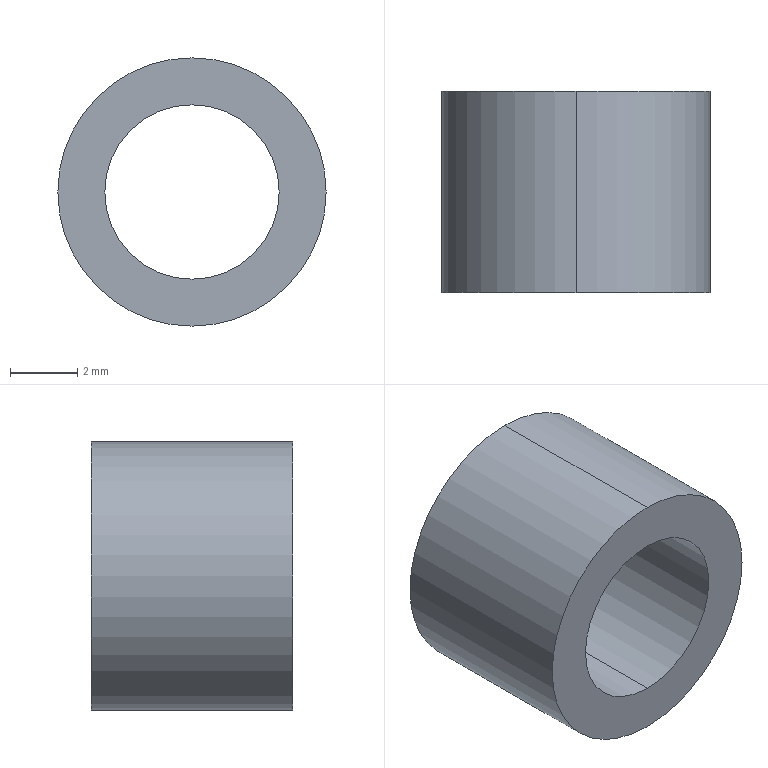Part | SolidWorks | features Extrusion 1 | 1 solid | 6 faces | box 8 x 6 x 8 mm | volume 174.17 mm3 | cylinder 4 | plane 2 | commonest cylinder face diameters 5.2 x2 8 x2
STEP:
#1=CARTESIAN_POINT('',(0.,6.,-2.6));
#2=VERTEX_POINT('',#1);
#3=CARTESIAN_POINT('',(0.,6.,2.6));
#4=VERTEX_POINT('',#3);
#5=CARTESIAN_POINT('',(0.,6.,0.));
#6=DIRECTION('',(0.,1.,0.));
#7=DIRECTION('',(0.,0.,1.));
#8=AXIS2_PLACEMENT_3D('',#5,#6,#7);
#9=CIRCLE('',#8,2.6);
#10=EDGE_CURVE('',#2,#4,#9,.T.);
#11=ORIENTED_EDGE('',*,*,#10,.T.);
#12=CARTESIAN_POINT('',(0.,0.,2.6));
#13=VERTEX_POINT('',#12);
#14=CARTESIAN_POINT('',(0.,6.,2.6));
#15=DIRECTION('',(0.,-1.,0.));
#16=VECTOR('',#15,1000.);
#17=LINE('',#14,#16);
#18=EDGE_CURVE('',#4,#13,#17,.T.);
#19=ORIENTED_EDGE('',*,*,#18,.T.);
#20=CARTESIAN_POINT('',(0.,0.,-2.6));
#21=VERTEX_POINT('',#20);
#22=CARTESIAN_POINT('',(0.,0.,0.));
#23=DIRECTION('',(0.,1.,0.));
#24=DIRECTION('',(0.,0.,1.));
#25=AXIS2_PLACEMENT_3D('',#22,#23,#24);
#26=CIRCLE('',#25,2.6);
#27=EDGE_CURVE('',#21,#13,#26,.T.);
#28=ORIENTED_EDGE('',*,*,#27,.F.);
#29=CARTESIAN_POINT('',(0.,6.,-2.6));
#30=DIRECTION('',(0.,-1.,0.));
#31=VECTOR('',#30,1000.);
#32=LINE('',#29,#31);
#33=EDGE_CURVE('',#2,#21,#32,.T.);
#34=ORIENTED_EDGE('',*,*,#33,.F.);
#35=EDGE_LOOP('',(#11,#19,#28,#34));
#36=FACE_OUTER_BOUND('',#35,.T.);
#37=CARTESIAN_POINT('',(0.,6.,0.));
#38=DIRECTION('',(0.,-1.,0.));
#39=DIRECTION('',(0.,0.,-1.));
#40=AXIS2_PLACEMENT_3D('',#37,#38,#39);
#41=CYLINDRICAL_SURFACE('',#40,2.6);
#42=ADVANCED_FACE('',(#36),#41,.F.);
#43=CARTESIAN_POINT('',(0.,6.,4.));
#44=VERTEX_POINT('',#43);
#45=CARTESIAN_POINT('',(0.,6.,-4.));
#46=VERTEX_POINT('',#45);
#47=CARTESIAN_POINT('',(0.,6.,0.));
#48=DIRECTION('',(0.,1.,0.));
#49=DIRECTION('',(0.,0.,1.));
#50=AXIS2_PLACEMENT_3D('',#47,#48,#49);
#51=CIRCLE('',#50,4.);
#52=EDGE_CURVE('',#44,#46,#51,.T.);
#53=ORIENTED_EDGE('',*,*,#52,.F.);
#54=CARTESIAN_POINT('',(0.,0.,4.));
#55=VERTEX_POINT('',#54);
#56=CARTESIAN_POINT('',(0.,6.,4.));
#57=DIRECTION('',(0.,-1.,0.));
#58=VECTOR('',#57,1000.);
#59=LINE('',#56,#58);
#60=EDGE_CURVE('',#44,#55,#59,.T.);
#61=ORIENTED_EDGE('',*,*,#60,.T.);
#62=CARTESIAN_POINT('',(0.,0.,-4.));
#63=VERTEX_POINT('',#62);
#64=CARTESIAN_POINT('',(0.,0.,0.));
#65=DIRECTION('',(0.,1.,0.));
#66=DIRECTION('',(0.,0.,1.));
#67=AXIS2_PLACEMENT_3D('',#64,#65,#66);
#68=CIRCLE('',#67,4.);
#69=EDGE_CURVE('',#55,#63,#68,.T.);
#70=ORIENTED_EDGE('',*,*,#69,.T.);
#71=CARTESIAN_POINT('',(0.,6.,-4.));
#72=DIRECTION('',(0.,-1.,0.));
#73=VECTOR('',#72,1000.);
#74=LINE('',#71,#73);
#75=EDGE_CURVE('',#46,#63,#74,.T.);
#76=ORIENTED_EDGE('',*,*,#75,.F.);
#77=EDGE_LOOP('',(#53,#61,#70,#76));
#78=FACE_OUTER_BOUND('',#77,.T.);
#79=CARTESIAN_POINT('',(0.,6.,0.));
#80=DIRECTION('',(0.,-1.,0.));
#81=DIRECTION('',(0.,0.,-1.));
#82=AXIS2_PLACEMENT_3D('',#79,#80,#81);
#83=CYLINDRICAL_SURFACE('',#82,4.);
#84=ADVANCED_FACE('',(#78),#83,.T.);
#85=CARTESIAN_POINT('',(0.,6.,0.));
#86=DIRECTION('',(0.,1.,0.));
#87=DIRECTION('',(0.,0.,1.));
#88=AXIS2_PLACEMENT_3D('',#85,#86,#87);
#89=CIRCLE('',#88,4.);
#90=EDGE_CURVE('',#46,#44,#89,.T.);
#91=ORIENTED_EDGE('',*,*,#90,.T.);
#92=ORIENTED_EDGE('',*,*,#52,.T.);
#93=EDGE_LOOP('',(#91,#92));
#94=FACE_OUTER_BOUND('',#93,.T.);
#95=ORIENTED_EDGE('',*,*,#10,.F.);
#96=CARTESIAN_POINT('',(0.,6.,0.));
#97=DIRECTION('',(0.,1.,0.));
#98=DIRECTION('',(0.,0.,1.));
#99=AXIS2_PLACEMENT_3D('',#96,#97,#98);
#100=CIRCLE('',#99,2.6);
#101=EDGE_CURVE('',#4,#2,#100,.T.);
#102=ORIENTED_EDGE('',*,*,#101,.F.);
#103=EDGE_LOOP('',(#95,#102));
#104=FACE_BOUND('',#103,.T.);
#105=CARTESIAN_POINT('',(0.,6.,0.));
#106=DIRECTION('',(0.,1.,0.));
#107=DIRECTION('',(0.,0.,1.));
#108=AXIS2_PLACEMENT_3D('',#105,#106,#107);
#109=PLANE('',#108);
#110=ADVANCED_FACE('',(#94,#104),#109,.T.);
#111=CARTESIAN_POINT('',(0.,0.,0.));
#112=DIRECTION('',(0.,1.,0.));
#113=DIRECTION('',(0.,0.,1.));
#114=AXIS2_PLACEMENT_3D('',#111,#112,#113);
#115=CIRCLE('',#114,4.);
#116=EDGE_CURVE('',#63,#55,#115,.T.);
#117=ORIENTED_EDGE('',*,*,#116,.F.);
#118=ORIENTED_EDGE('',*,*,#69,.F.);
#119=EDGE_LOOP('',(#117,#118));
#120=FACE_OUTER_BOUND('',#119,.T.);
#121=ORIENTED_EDGE('',*,*,#27,.T.);
#122=CARTESIAN_POINT('',(0.,0.,0.));
#123=DIRECTION('',(0.,1.,0.));
#124=DIRECTION('',(0.,0.,1.));
#125=AXIS2_PLACEMENT_3D('',#122,#123,#124);
#126=CIRCLE('',#125,2.6);
#127=EDGE_CURVE('',#13,#21,#126,.T.);
#128=ORIENTED_EDGE('',*,*,#127,.T.);
#129=EDGE_LOOP('',(#121,#128));
#130=FACE_BOUND('',#129,.T.);
#131=CARTESIAN_POINT('',(0.,0.,0.));
#132=DIRECTION('',(0.,1.,0.));
#133=DIRECTION('',(0.,0.,1.));
#134=AXIS2_PLACEMENT_3D('',#131,#132,#133);
#135=PLANE('',#134);
#136=ADVANCED_FACE('',(#120,#130),#135,.F.);
#137=ORIENTED_EDGE('',*,*,#60,.F.);
#138=ORIENTED_EDGE('',*,*,#90,.F.);
#139=ORIENTED_EDGE('',*,*,#75,.T.);
#140=ORIENTED_EDGE('',*,*,#116,.T.);
#141=EDGE_LOOP('',(#137,#138,#139,#140));
#142=FACE_OUTER_BOUND('',#141,.T.);
#143=CARTESIAN_POINT('',(0.,6.,0.));
#144=DIRECTION('',(0.,-1.,0.));
#145=DIRECTION('',(0.,0.,-1.));
#146=AXIS2_PLACEMENT_3D('',#143,#144,#145);
#147=CYLINDRICAL_SURFACE('',#146,4.);
#148=ADVANCED_FACE('',(#142),#147,.T.);
#149=ORIENTED_EDGE('',*,*,#18,.F.);
#150=ORIENTED_EDGE('',*,*,#101,.T.);
#151=ORIENTED_EDGE('',*,*,#33,.T.);
#152=ORIENTED_EDGE('',*,*,#127,.F.);
#153=EDGE_LOOP('',(#149,#150,#151,#152));
#154=FACE_OUTER_BOUND('',#153,.T.);
#155=CARTESIAN_POINT('',(0.,6.,0.));
#156=DIRECTION('',(0.,-1.,0.));
#157=DIRECTION('',(0.,0.,-1.));
#158=AXIS2_PLACEMENT_3D('',#155,#156,#157);
#159=CYLINDRICAL_SURFACE('',#158,2.6);
#160=ADVANCED_FACE('',(#154),#159,.F.);
#161=CLOSED_SHELL('',(#42,#84,#110,#136,#148,#160));
#162=MANIFOLD_SOLID_BREP('',#161);
#163=CARTESIAN_POINT('',(0.,0.,0.));
#164=DIRECTION('',(0.,0.,1.));
#165=DIRECTION('',(1.,0.,0.));
#166=AXIS2_PLACEMENT_3D('',#163,#164,#165);
#167=(LENGTH_UNIT()NAMED_UNIT(*)SI_UNIT(.MILLI.,.METRE.));
#168=UNCERTAINTY_MEASURE_WITH_UNIT(LENGTH_MEASURE(0.00001),#167,'','');
#169=(NAMED_UNIT(*)PLANE_ANGLE_UNIT()SI_UNIT($,.RADIAN.));
#170=(NAMED_UNIT(*)SI_UNIT($,.STERADIAN.)SOLID_ANGLE_UNIT());
#171=(GEOMETRIC_REPRESENTATION_CONTEXT(3)GLOBAL_UNCERTAINTY_ASSIGNED_CONTEXT((#168))GLOBAL_UNIT_ASSIGNED_CONTEXT((#167,#169,#170))REPRESENTATION_CONTEXT('',''));
#172=ADVANCED_BREP_SHAPE_REPRESENTATION('',(#162,#166),#171);